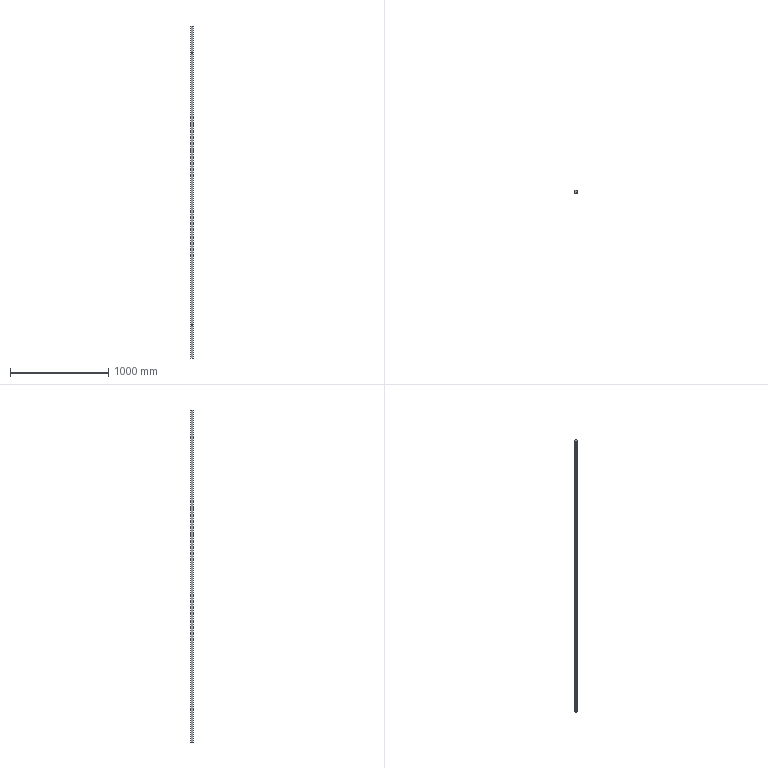Part | STEP file | BCC3 H16_8 | 1 solid | 14 faces | box 25 x 25 x 3385 mm | volume 2110006 mm3 | plane 10 | cylinder 4 | commonest cylinder face diameters 10 x4
STEP:
#1=CARTESIAN_POINT('',(0.,0.,0.));
#2=DIRECTION('',(0.,0.,1.));
#3=DIRECTION('',(1.,0.,0.));
#4=AXIS2_PLACEMENT_3D('',#1,#2,#3);
#5=CARTESIAN_POINT('',(0.,-12.5,-1347.5));
#6=VERTEX_POINT('',#5);
#7=CARTESIAN_POINT('',(0.,12.5,-1347.5));
#8=VERTEX_POINT('',#7);
#9=CARTESIAN_POINT('',(0.,-12.5,-1347.5));
#10=DIRECTION('',(0.,1.,0.));
#11=VECTOR('',#10,1.);
#12=LINE('',#9,#11);
#13=CARTESIAN_POINT('',(0.,-12.5,-1352.5));
#14=DIRECTION('',(0.,1.,0.));
#15=DIRECTION('',(0.,0.,1.));
#16=AXIS2_PLACEMENT_3D('',#13,#14,#15);
#17=CYLINDRICAL_SURFACE('',#16,5.);
#18=CARTESIAN_POINT('',(6.283,0.));
#19=DIRECTION('',(0.,1.));
#20=VECTOR('',#19,1.);
#21=LINE('',#18,#20);
#22=(GEOMETRIC_REPRESENTATION_CONTEXT(2)PARAMETRIC_REPRESENTATION_CONTEXT()REPRESENTATION_CONTEXT('',''));
#23=DEFINITIONAL_REPRESENTATION('',(#21),#22);
#24=PCURVE('',#17,#23);
#25=CARTESIAN_POINT('',(0.,-12.5,-1352.5));
#26=DIRECTION('',(0.,1.,0.));
#27=DIRECTION('',(0.,0.,1.));
#28=AXIS2_PLACEMENT_3D('',#25,#26,#27);
#29=CYLINDRICAL_SURFACE('',#28,5.);
#30=CARTESIAN_POINT('',(0.,0.));
#31=DIRECTION('',(0.,1.));
#32=VECTOR('',#31,1.);
#33=LINE('',#30,#32);
#34=(GEOMETRIC_REPRESENTATION_CONTEXT(2)PARAMETRIC_REPRESENTATION_CONTEXT()REPRESENTATION_CONTEXT('',''));
#35=DEFINITIONAL_REPRESENTATION('',(#33),#34);
#36=PCURVE('',#29,#35);
#37=SURFACE_CURVE('',#12,(#24,#36),.PCURVE_S1.);
#38=EDGE_CURVE('',#6,#8,#37,.T.);
#39=ORIENTED_EDGE('',*,*,#38,.T.);
#40=CARTESIAN_POINT('',(0.,12.5,-1357.5));
#41=VERTEX_POINT('',#40);
#42=CARTESIAN_POINT('',(0.,12.5,-1352.5));
#43=DIRECTION('',(0.,1.,0.));
#44=DIRECTION('',(0.,0.,1.));
#45=AXIS2_PLACEMENT_3D('',#42,#43,#44);
#46=CIRCLE('',#45,5.);
#47=CARTESIAN_POINT('',(0.,25.));
#48=DIRECTION('',(1.,0.));
#49=VECTOR('',#48,1.);
#50=LINE('',#47,#49);
#51=(GEOMETRIC_REPRESENTATION_CONTEXT(2)PARAMETRIC_REPRESENTATION_CONTEXT()REPRESENTATION_CONTEXT('',''));
#52=DEFINITIONAL_REPRESENTATION('',(#50),#51);
#53=PCURVE('',#17,#52);
#54=CARTESIAN_POINT('',(-12.5,12.5,1692.5));
#55=DIRECTION('',(0.,-1.,0.));
#56=DIRECTION('',(0.,0.,-1.));
#57=AXIS2_PLACEMENT_3D('',#54,#55,#56);
#58=PLANE('',#57);
#59=CARTESIAN_POINT('',(3040.,12.5));
#60=CARTESIAN_POINT('',(3040.,21.16));
#61=CARTESIAN_POINT('',(3047.5,16.83));
#62=CARTESIAN_POINT('',(3055.,12.5));
#63=CARTESIAN_POINT('',(3047.5,8.17));
#64=CARTESIAN_POINT('',(3040.,3.84));
#65=CARTESIAN_POINT('',(3040.,12.5));
#66=(BOUNDED_CURVE()B_SPLINE_CURVE(2,(#59,#60,#61,#62,#63,#64,#65),.UNSPECIFIED.,.T.,.F.)B_SPLINE_CURVE_WITH_KNOTS((1,2,2,2,2,1),(-2.094,0.,2.094,4.189,6.283,8.378),.UNSPECIFIED.)CURVE()GEOMETRIC_REPRESENTATION_ITEM()RATIONAL_B_SPLINE_CURVE((1.,0.5,1.,0.5,1.,0.5,1.))REPRESENTATION_ITEM(''));
#67=(GEOMETRIC_REPRESENTATION_CONTEXT(2)PARAMETRIC_REPRESENTATION_CONTEXT()REPRESENTATION_CONTEXT('',''));
#68=DEFINITIONAL_REPRESENTATION('',(#66),#67);
#69=PCURVE('',#58,#68);
#70=SURFACE_CURVE('',#46,(#53,#69),.PCURVE_S1.);
#71=EDGE_CURVE('',#41,#8,#70,.T.);
#72=ORIENTED_EDGE('',*,*,#71,.F.);
#73=CARTESIAN_POINT('',(0.,-12.5,-1357.5));
#74=VERTEX_POINT('',#73);
#75=CARTESIAN_POINT('',(0.,-12.5,-1357.5));
#76=DIRECTION('',(0.,1.,0.));
#77=VECTOR('',#76,1.);
#78=LINE('',#75,#77);
#79=CARTESIAN_POINT('',(3.142,0.));
#80=DIRECTION('',(0.,1.));
#81=VECTOR('',#80,1.);
#82=LINE('',#79,#81);
#83=(GEOMETRIC_REPRESENTATION_CONTEXT(2)PARAMETRIC_REPRESENTATION_CONTEXT()REPRESENTATION_CONTEXT('',''));
#84=DEFINITIONAL_REPRESENTATION('',(#82),#83);
#85=PCURVE('',#17,#84);
#86=CARTESIAN_POINT('',(3.142,0.));
#87=DIRECTION('',(0.,1.));
#88=VECTOR('',#87,1.);
#89=LINE('',#86,#88);
#90=(GEOMETRIC_REPRESENTATION_CONTEXT(2)PARAMETRIC_REPRESENTATION_CONTEXT()REPRESENTATION_CONTEXT('',''));
#91=DEFINITIONAL_REPRESENTATION('',(#89),#90);
#92=PCURVE('',#29,#91);
#93=SURFACE_CURVE('',#78,(#85,#92),.PCURVE_S1.);
#94=EDGE_CURVE('',#74,#41,#93,.T.);
#95=ORIENTED_EDGE('',*,*,#94,.F.);
#96=CARTESIAN_POINT('',(0.,-12.5,-1352.5));
#97=DIRECTION('',(0.,1.,0.));
#98=DIRECTION('',(0.,0.,1.));
#99=AXIS2_PLACEMENT_3D('',#96,#97,#98);
#100=CIRCLE('',#99,5.);
#101=CARTESIAN_POINT('',(0.,0.));
#102=DIRECTION('',(1.,0.));
#103=VECTOR('',#102,1.);
#104=LINE('',#101,#103);
#105=(GEOMETRIC_REPRESENTATION_CONTEXT(2)PARAMETRIC_REPRESENTATION_CONTEXT()REPRESENTATION_CONTEXT('',''));
#106=DEFINITIONAL_REPRESENTATION('',(#104),#105);
#107=PCURVE('',#17,#106);
#108=CARTESIAN_POINT('',(-12.5,-12.5,1692.5));
#109=DIRECTION('',(0.,1.,0.));
#110=DIRECTION('',(-1.,0.,0.));
#111=AXIS2_PLACEMENT_3D('',#108,#109,#110);
#112=PLANE('',#111);
#113=CARTESIAN_POINT('',(-12.5,-3045.));
#114=DIRECTION('',(0.,1.));
#115=AXIS2_PLACEMENT_2D('',#113,#114);
#116=CIRCLE('',#115,5.);
#117=(GEOMETRIC_REPRESENTATION_CONTEXT(2)PARAMETRIC_REPRESENTATION_CONTEXT()REPRESENTATION_CONTEXT('',''));
#118=DEFINITIONAL_REPRESENTATION('',(#116),#117);
#119=PCURVE('',#112,#118);
#120=SURFACE_CURVE('',#100,(#107,#119),.PCURVE_S1.);
#121=EDGE_CURVE('',#74,#6,#120,.T.);
#122=ORIENTED_EDGE('',*,*,#121,.T.);
#123=EDGE_LOOP('',(#39,#72,#95,#122));
#124=FACE_BOUND('',#123,.F.);
#125=ADVANCED_FACE('',(#124),#17,.F.);
#126=CARTESIAN_POINT('',(0.,-12.5,1422.5));
#127=VERTEX_POINT('',#126);
#128=CARTESIAN_POINT('',(0.,12.5,1422.5));
#129=VERTEX_POINT('',#128);
#130=CARTESIAN_POINT('',(0.,-12.5,1422.5));
#131=DIRECTION('',(0.,1.,0.));
#132=VECTOR('',#131,1.);
#133=LINE('',#130,#132);
#134=CARTESIAN_POINT('',(0.,-12.5,1417.5));
#135=DIRECTION('',(0.,1.,0.));
#136=DIRECTION('',(0.,0.,1.));
#137=AXIS2_PLACEMENT_3D('',#134,#135,#136);
#138=CYLINDRICAL_SURFACE('',#137,5.);
#139=CARTESIAN_POINT('',(6.283,0.));
#140=DIRECTION('',(0.,1.));
#141=VECTOR('',#140,1.);
#142=LINE('',#139,#141);
#143=(GEOMETRIC_REPRESENTATION_CONTEXT(2)PARAMETRIC_REPRESENTATION_CONTEXT()REPRESENTATION_CONTEXT('',''));
#144=DEFINITIONAL_REPRESENTATION('',(#142),#143);
#145=PCURVE('',#138,#144);
#146=CARTESIAN_POINT('',(0.,-12.5,1417.5));
#147=DIRECTION('',(0.,1.,0.));
#148=DIRECTION('',(0.,0.,1.));
#149=AXIS2_PLACEMENT_3D('',#146,#147,#148);
#150=CYLINDRICAL_SURFACE('',#149,5.);
#151=CARTESIAN_POINT('',(0.,0.));
#152=DIRECTION('',(0.,1.));
#153=VECTOR('',#152,1.);
#154=LINE('',#151,#153);
#155=(GEOMETRIC_REPRESENTATION_CONTEXT(2)PARAMETRIC_REPRESENTATION_CONTEXT()REPRESENTATION_CONTEXT('',''));
#156=DEFINITIONAL_REPRESENTATION('',(#154),#155);
#157=PCURVE('',#150,#156);
#158=SURFACE_CURVE('',#133,(#145,#157),.PCURVE_S1.);
#159=EDGE_CURVE('',#127,#129,#158,.T.);
#160=ORIENTED_EDGE('',*,*,#159,.T.);
#161=CARTESIAN_POINT('',(0.,12.5,1412.5));
#162=VERTEX_POINT('',#161);
#163=CARTESIAN_POINT('',(0.,12.5,1417.5));
#164=DIRECTION('',(0.,1.,0.));
#165=DIRECTION('',(0.,0.,1.));
#166=AXIS2_PLACEMENT_3D('',#163,#164,#165);
#167=CIRCLE('',#166,5.);
#168=CARTESIAN_POINT('',(0.,25.));
#169=DIRECTION('',(1.,0.));
#170=VECTOR('',#169,1.);
#171=LINE('',#168,#170);
#172=(GEOMETRIC_REPRESENTATION_CONTEXT(2)PARAMETRIC_REPRESENTATION_CONTEXT()REPRESENTATION_CONTEXT('',''));
#173=DEFINITIONAL_REPRESENTATION('',(#171),#172);
#174=PCURVE('',#138,#173);
#175=CARTESIAN_POINT('',(270.,12.5));
#176=CARTESIAN_POINT('',(270.,21.16));
#177=CARTESIAN_POINT('',(277.5,16.83));
#178=CARTESIAN_POINT('',(285.,12.5));
#179=CARTESIAN_POINT('',(277.5,8.17));
#180=CARTESIAN_POINT('',(270.,3.84));
#181=CARTESIAN_POINT('',(270.,12.5));
#182=(BOUNDED_CURVE()B_SPLINE_CURVE(2,(#175,#176,#177,#178,#179,#180,#181),.UNSPECIFIED.,.T.,.F.)B_SPLINE_CURVE_WITH_KNOTS((1,2,2,2,2,1),(-2.094,0.,2.094,4.189,6.283,8.378),.UNSPECIFIED.)CURVE()GEOMETRIC_REPRESENTATION_ITEM()RATIONAL_B_SPLINE_CURVE((1.,0.5,1.,0.5,1.,0.5,1.))REPRESENTATION_ITEM(''));
#183=(GEOMETRIC_REPRESENTATION_CONTEXT(2)PARAMETRIC_REPRESENTATION_CONTEXT()REPRESENTATION_CONTEXT('',''));
#184=DEFINITIONAL_REPRESENTATION('',(#182),#183);
#185=PCURVE('',#58,#184);
#186=SURFACE_CURVE('',#167,(#174,#185),.PCURVE_S1.);
#187=EDGE_CURVE('',#162,#129,#186,.T.);
#188=ORIENTED_EDGE('',*,*,#187,.F.);
#189=CARTESIAN_POINT('',(0.,-12.5,1412.5));
#190=VERTEX_POINT('',#189);
#191=CARTESIAN_POINT('',(0.,-12.5,1412.5));
#192=DIRECTION('',(0.,1.,0.));
#193=VECTOR('',#192,1.);
#194=LINE('',#191,#193);
#195=CARTESIAN_POINT('',(3.142,0.));
#196=DIRECTION('',(0.,1.));
#197=VECTOR('',#196,1.);
#198=LINE('',#195,#197);
#199=(GEOMETRIC_REPRESENTATION_CONTEXT(2)PARAMETRIC_REPRESENTATION_CONTEXT()REPRESENTATION_CONTEXT('',''));
#200=DEFINITIONAL_REPRESENTATION('',(#198),#199);
#201=PCURVE('',#138,#200);
#202=CARTESIAN_POINT('',(3.142,0.));
#203=DIRECTION('',(0.,1.));
#204=VECTOR('',#203,1.);
#205=LINE('',#202,#204);
#206=(GEOMETRIC_REPRESENTATION_CONTEXT(2)PARAMETRIC_REPRESENTATION_CONTEXT()REPRESENTATION_CONTEXT('',''));
#207=DEFINITIONAL_REPRESENTATION('',(#205),#206);
#208=PCURVE('',#150,#207);
#209=SURFACE_CURVE('',#194,(#201,#208),.PCURVE_S1.);
#210=EDGE_CURVE('',#190,#162,#209,.T.);
#211=ORIENTED_EDGE('',*,*,#210,.F.);
#212=CARTESIAN_POINT('',(0.,-12.5,1417.5));
#213=DIRECTION('',(0.,1.,0.));
#214=DIRECTION('',(0.,0.,1.));
#215=AXIS2_PLACEMENT_3D('',#212,#213,#214);
#216=CIRCLE('',#215,5.);
#217=CARTESIAN_POINT('',(0.,0.));
#218=DIRECTION('',(1.,0.));
#219=VECTOR('',#218,1.);
#220=LINE('',#217,#219);
#221=(GEOMETRIC_REPRESENTATION_CONTEXT(2)PARAMETRIC_REPRESENTATION_CONTEXT()REPRESENTATION_CONTEXT('',''));
#222=DEFINITIONAL_REPRESENTATION('',(#220),#221);
#223=PCURVE('',#138,#222);
#224=CARTESIAN_POINT('',(-12.5,-275.));
#225=DIRECTION('',(0.,1.));
#226=AXIS2_PLACEMENT_2D('',#224,#225);
#227=CIRCLE('',#226,5.);
#228=(GEOMETRIC_REPRESENTATION_CONTEXT(2)PARAMETRIC_REPRESENTATION_CONTEXT()REPRESENTATION_CONTEXT('',''));
#229=DEFINITIONAL_REPRESENTATION('',(#227),#228);
#230=PCURVE('',#112,#229);
#231=SURFACE_CURVE('',#216,(#223,#230),.PCURVE_S1.);
#232=EDGE_CURVE('',#190,#127,#231,.T.);
#233=ORIENTED_EDGE('',*,*,#232,.T.);
#234=EDGE_LOOP('',(#160,#188,#211,#233));
#235=FACE_BOUND('',#234,.F.);
#236=ADVANCED_FACE('',(#235),#138,.F.);
#237=CARTESIAN_POINT('',(-12.5,12.,-1692.5));
#238=VERTEX_POINT('',#237);
#239=CARTESIAN_POINT('',(-12.5,-12.,-1692.5));
#240=VERTEX_POINT('',#239);
#241=CARTESIAN_POINT('',(-12.5,12.5,-1692.5));
#242=DIRECTION('',(0.,-1.,0.));
#243=VECTOR('',#242,1.);
#244=LINE('',#241,#243);
#245=CARTESIAN_POINT('',(-12.5,12.5,1692.5));
#246=DIRECTION('',(1.,0.,0.));
#247=DIRECTION('',(0.,1.,0.));
#248=AXIS2_PLACEMENT_3D('',#245,#246,#247);
#249=PLANE('',#248);
#250=CARTESIAN_POINT('',(0.,-3385.));
#251=DIRECTION('',(-1.,0.));
#252=VECTOR('',#251,1.);
#253=LINE('',#250,#252);
#254=(GEOMETRIC_REPRESENTATION_CONTEXT(2)PARAMETRIC_REPRESENTATION_CONTEXT()REPRESENTATION_CONTEXT('',''));
#255=DEFINITIONAL_REPRESENTATION('',(#253),#254);
#256=PCURVE('',#249,#255);
#257=CARTESIAN_POINT('',(0.,0.,-1692.5));
#258=DIRECTION('',(0.,0.,1.));
#259=DIRECTION('',(1.,0.,0.));
#260=AXIS2_PLACEMENT_3D('',#257,#258,#259);
#261=PLANE('',#260);
#262=CARTESIAN_POINT('',(-12.5,12.5));
#263=DIRECTION('',(0.,-1.));
#264=VECTOR('',#263,1.);
#265=LINE('',#262,#264);
#266=(GEOMETRIC_REPRESENTATION_CONTEXT(2)PARAMETRIC_REPRESENTATION_CONTEXT()REPRESENTATION_CONTEXT('',''));
#267=DEFINITIONAL_REPRESENTATION('',(#265),#266);
#268=PCURVE('',#261,#267);
#269=SURFACE_CURVE('',#244,(#256,#268),.PCURVE_S1.);
#270=EDGE_CURVE('',#238,#240,#269,.T.);
#271=ORIENTED_EDGE('',*,*,#270,.T.);
#272=CARTESIAN_POINT('',(-12.5,-12.,1692.5));
#273=VERTEX_POINT('',#272);
#274=CARTESIAN_POINT('',(-12.5,-12.,1692.5));
#275=DIRECTION('',(0.,0.,1.));
#276=VECTOR('',#275,1.);
#277=LINE('',#274,#276);
#278=CARTESIAN_POINT('',(-24.5,0.));
#279=DIRECTION('',(0.,1.));
#280=VECTOR('',#279,1.);
#281=LINE('',#278,#280);
#282=(GEOMETRIC_REPRESENTATION_CONTEXT(2)PARAMETRIC_REPRESENTATION_CONTEXT()REPRESENTATION_CONTEXT('',''));
#283=DEFINITIONAL_REPRESENTATION('',(#281),#282);
#284=PCURVE('',#249,#283);
#285=CARTESIAN_POINT('',(-12.,-12.5,1692.5));
#286=DIRECTION('',(0.7071,0.7071,0.));
#287=DIRECTION('',(0.,0.,-1.));
#288=AXIS2_PLACEMENT_3D('',#285,#286,#287);
#289=PLANE('',#288);
#290=CARTESIAN_POINT('',(0.,0.7071));
#291=DIRECTION('',(-1.,0.));
#292=VECTOR('',#291,1.);
#293=LINE('',#290,#292);
#294=(GEOMETRIC_REPRESENTATION_CONTEXT(2)PARAMETRIC_REPRESENTATION_CONTEXT()REPRESENTATION_CONTEXT('',''));
#295=DEFINITIONAL_REPRESENTATION('',(#293),#294);
#296=PCURVE('',#289,#295);
#297=SURFACE_CURVE('',#277,(#284,#296),.PCURVE_S1.);
#298=EDGE_CURVE('',#240,#273,#297,.T.);
#299=ORIENTED_EDGE('',*,*,#298,.T.);
#300=CARTESIAN_POINT('',(-12.5,12.,1692.5));
#301=VERTEX_POINT('',#300);
#302=CARTESIAN_POINT('',(-12.5,12.5,1692.5));
#303=DIRECTION('',(0.,-1.,0.));
#304=VECTOR('',#303,1.);
#305=LINE('',#302,#304);
#306=CARTESIAN_POINT('',(0.,0.));
#307=DIRECTION('',(-1.,0.));
#308=VECTOR('',#307,1.);
#309=LINE('',#306,#308);
#310=(GEOMETRIC_REPRESENTATION_CONTEXT(2)PARAMETRIC_REPRESENTATION_CONTEXT()REPRESENTATION_CONTEXT('',''));
#311=DEFINITIONAL_REPRESENTATION('',(#309),#310);
#312=PCURVE('',#249,#311);
#313=CARTESIAN_POINT('',(0.,0.,1692.5));
#314=DIRECTION('',(0.,0.,1.));
#315=DIRECTION('',(1.,0.,0.));
#316=AXIS2_PLACEMENT_3D('',#313,#314,#315);
#317=PLANE('',#316);
#318=CARTESIAN_POINT('',(-12.5,12.5));
#319=DIRECTION('',(0.,-1.));
#320=VECTOR('',#319,1.);
#321=LINE('',#318,#320);
#322=(GEOMETRIC_REPRESENTATION_CONTEXT(2)PARAMETRIC_REPRESENTATION_CONTEXT()REPRESENTATION_CONTEXT('',''));
#323=DEFINITIONAL_REPRESENTATION('',(#321),#322);
#324=PCURVE('',#317,#323);
#325=SURFACE_CURVE('',#305,(#312,#324),.PCURVE_S1.);
#326=EDGE_CURVE('',#301,#273,#325,.T.);
#327=ORIENTED_EDGE('',*,*,#326,.F.);
#328=CARTESIAN_POINT('',(-12.5,12.,1692.5));
#329=DIRECTION('',(0.,0.,-1.));
#330=VECTOR('',#329,1.);
#331=LINE('',#328,#330);
#332=CARTESIAN_POINT('',(-0.5,0.));
#333=DIRECTION('',(0.,-1.));
#334=VECTOR('',#333,1.);
#335=LINE('',#332,#334);
#336=(GEOMETRIC_REPRESENTATION_CONTEXT(2)PARAMETRIC_REPRESENTATION_CONTEXT()REPRESENTATION_CONTEXT('',''));
#337=DEFINITIONAL_REPRESENTATION('',(#335),#336);
#338=PCURVE('',#249,#337);
#339=CARTESIAN_POINT('',(-12.5,12.,1692.5));
#340=DIRECTION('',(0.7071,-0.7071,0.));
#341=DIRECTION('',(0.,0.,-1.));
#342=AXIS2_PLACEMENT_3D('',#339,#340,#341);
#343=PLANE('',#342);
#344=CARTESIAN_POINT('',(0.,0.));
#345=DIRECTION('',(1.,0.));
#346=VECTOR('',#345,1.);
#347=LINE('',#344,#346);
#348=(GEOMETRIC_REPRESENTATION_CONTEXT(2)PARAMETRIC_REPRESENTATION_CONTEXT()REPRESENTATION_CONTEXT('',''));
#349=DEFINITIONAL_REPRESENTATION('',(#347),#348);
#350=PCURVE('',#343,#349);
#351=SURFACE_CURVE('',#331,(#338,#350),.PCURVE_S1.);
#352=EDGE_CURVE('',#301,#238,#351,.T.);
#353=ORIENTED_EDGE('',*,*,#352,.T.);
#354=EDGE_LOOP('',(#271,#299,#327,#353));
#355=FACE_BOUND('',#354,.T.);
#356=ADVANCED_FACE('',(#355),#249,.F.);
#357=CARTESIAN_POINT('',(0.,-12.5,-1352.5));
#358=DIRECTION('',(0.,1.,0.));
#359=DIRECTION('',(0.,0.,1.));
#360=AXIS2_PLACEMENT_3D('',#357,#358,#359);
#361=CIRCLE('',#360,5.);
#362=CARTESIAN_POINT('',(-12.5,-3045.));
#363=DIRECTION('',(0.,1.));
#364=AXIS2_PLACEMENT_2D('',#362,#363);
#365=CIRCLE('',#364,5.);
#366=(GEOMETRIC_REPRESENTATION_CONTEXT(2)PARAMETRIC_REPRESENTATION_CONTEXT()REPRESENTATION_CONTEXT('',''));
#367=DEFINITIONAL_REPRESENTATION('',(#365),#366);
#368=PCURVE('',#112,#367);
#369=CARTESIAN_POINT('',(0.,0.));
#370=DIRECTION('',(1.,0.));
#371=VECTOR('',#370,1.);
#372=LINE('',#369,#371);
#373=(GEOMETRIC_REPRESENTATION_CONTEXT(2)PARAMETRIC_REPRESENTATION_CONTEXT()REPRESENTATION_CONTEXT('',''));
#374=DEFINITIONAL_REPRESENTATION('',(#372),#373);
#375=PCURVE('',#29,#374);
#376=SURFACE_CURVE('',#361,(#368,#375),.PCURVE_S1.);
#377=EDGE_CURVE('',#6,#74,#376,.T.);
#378=ORIENTED_EDGE('',*,*,#377,.T.);
#379=ORIENTED_EDGE('',*,*,#121,.T.);
#380=EDGE_LOOP('',(#378,#379));
#381=FACE_BOUND('',#380,.T.);
#382=CARTESIAN_POINT('',(0.,-12.5,1417.5));
#383=DIRECTION('',(0.,1.,0.));
#384=DIRECTION('',(0.,0.,1.));
#385=AXIS2_PLACEMENT_3D('',#382,#383,#384);
#386=CIRCLE('',#385,5.);
#387=CARTESIAN_POINT('',(-12.5,-275.));
#388=DIRECTION('',(0.,1.));
#389=AXIS2_PLACEMENT_2D('',#387,#388);
#390=CIRCLE('',#389,5.);
#391=(GEOMETRIC_REPRESENTATION_CONTEXT(2)PARAMETRIC_REPRESENTATION_CONTEXT()REPRESENTATION_CONTEXT('',''));
#392=DEFINITIONAL_REPRESENTATION('',(#390),#391);
#393=PCURVE('',#112,#392);
#394=CARTESIAN_POINT('',(0.,0.));
#395=DIRECTION('',(1.,0.));
#396=VECTOR('',#395,1.);
#397=LINE('',#394,#396);
#398=(GEOMETRIC_REPRESENTATION_CONTEXT(2)PARAMETRIC_REPRESENTATION_CONTEXT()REPRESENTATION_CONTEXT('',''));
#399=DEFINITIONAL_REPRESENTATION('',(#397),#398);
#400=PCURVE('',#150,#399);
#401=SURFACE_CURVE('',#386,(#393,#400),.PCURVE_S1.);
#402=EDGE_CURVE('',#127,#190,#401,.T.);
#403=ORIENTED_EDGE('',*,*,#402,.T.);
#404=ORIENTED_EDGE('',*,*,#232,.T.);
#405=EDGE_LOOP('',(#403,#404));
#406=FACE_BOUND('',#405,.T.);
#407=CARTESIAN_POINT('',(-12.,-12.5,1692.5));
#408=VERTEX_POINT('',#407);
#409=CARTESIAN_POINT('',(12.,-12.5,1692.5));
#410=VERTEX_POINT('',#409);
#411=CARTESIAN_POINT('',(-12.5,-12.5,1692.5));
#412=DIRECTION('',(1.,0.,0.));
#413=VECTOR('',#412,1.);
#414=LINE('',#411,#413);
#415=CARTESIAN_POINT('',(0.,0.));
#416=DIRECTION('',(-1.,0.));
#417=VECTOR('',#416,1.);
#418=LINE('',#415,#417);
#419=(GEOMETRIC_REPRESENTATION_CONTEXT(2)PARAMETRIC_REPRESENTATION_CONTEXT()REPRESENTATION_CONTEXT('',''));
#420=DEFINITIONAL_REPRESENTATION('',(#418),#419);
#421=PCURVE('',#112,#420);
#422=CARTESIAN_POINT('',(-12.5,-12.5));
#423=DIRECTION('',(1.,0.));
#424=VECTOR('',#423,1.);
#425=LINE('',#422,#424);
#426=(GEOMETRIC_REPRESENTATION_CONTEXT(2)PARAMETRIC_REPRESENTATION_CONTEXT()REPRESENTATION_CONTEXT('',''));
#427=DEFINITIONAL_REPRESENTATION('',(#425),#426);
#428=PCURVE('',#317,#427);
#429=SURFACE_CURVE('',#414,(#421,#428),.PCURVE_S1.);
#430=EDGE_CURVE('',#408,#410,#429,.T.);
#431=ORIENTED_EDGE('',*,*,#430,.F.);
#432=CARTESIAN_POINT('',(-12.,-12.5,-1692.5));
#433=VERTEX_POINT('',#432);
#434=CARTESIAN_POINT('',(-12.,-12.5,1692.5));
#435=DIRECTION('',(0.,0.,-1.));
#436=VECTOR('',#435,1.);
#437=LINE('',#434,#436);
#438=CARTESIAN_POINT('',(-0.5,0.));
#439=DIRECTION('',(0.,-1.));
#440=VECTOR('',#439,1.);
#441=LINE('',#438,#440);
#442=(GEOMETRIC_REPRESENTATION_CONTEXT(2)PARAMETRIC_REPRESENTATION_CONTEXT()REPRESENTATION_CONTEXT('',''));
#443=DEFINITIONAL_REPRESENTATION('',(#441),#442);
#444=PCURVE('',#112,#443);
#445=CARTESIAN_POINT('',(0.,0.));
#446=DIRECTION('',(1.,0.));
#447=VECTOR('',#446,1.);
#448=LINE('',#445,#447);
#449=(GEOMETRIC_REPRESENTATION_CONTEXT(2)PARAMETRIC_REPRESENTATION_CONTEXT()REPRESENTATION_CONTEXT('',''));
#450=DEFINITIONAL_REPRESENTATION('',(#448),#449);
#451=PCURVE('',#289,#450);
#452=SURFACE_CURVE('',#437,(#444,#451),.PCURVE_S1.);
#453=EDGE_CURVE('',#408,#433,#452,.T.);
#454=ORIENTED_EDGE('',*,*,#453,.T.);
#455=CARTESIAN_POINT('',(12.,-12.5,-1692.5));
#456=VERTEX_POINT('',#455);
#457=CARTESIAN_POINT('',(-12.5,-12.5,-1692.5));
#458=DIRECTION('',(1.,0.,0.));
#459=VECTOR('',#458,1.);
#460=LINE('',#457,#459);
#461=CARTESIAN_POINT('',(0.,-3385.));
#462=DIRECTION('',(-1.,0.));
#463=VECTOR('',#462,1.);
#464=LINE('',#461,#463);
#465=(GEOMETRIC_REPRESENTATION_CONTEXT(2)PARAMETRIC_REPRESENTATION_CONTEXT()REPRESENTATION_CONTEXT('',''));
#466=DEFINITIONAL_REPRESENTATION('',(#464),#465);
#467=PCURVE('',#112,#466);
#468=CARTESIAN_POINT('',(-12.5,-12.5));
#469=DIRECTION('',(1.,0.));
#470=VECTOR('',#469,1.);
#471=LINE('',#468,#470);
#472=(GEOMETRIC_REPRESENTATION_CONTEXT(2)PARAMETRIC_REPRESENTATION_CONTEXT()REPRESENTATION_CONTEXT('',''));
#473=DEFINITIONAL_REPRESENTATION('',(#471),#472);
#474=PCURVE('',#261,#473);
#475=SURFACE_CURVE('',#460,(#467,#474),.PCURVE_S1.);
#476=EDGE_CURVE('',#433,#456,#475,.T.);
#477=ORIENTED_EDGE('',*,*,#476,.T.);
#478=CARTESIAN_POINT('',(12.,-12.5,1692.5));
#479=DIRECTION('',(0.,0.,1.));
#480=VECTOR('',#479,1.);
#481=LINE('',#478,#480);
#482=CARTESIAN_POINT('',(-24.5,0.));
#483=DIRECTION('',(0.,1.));
#484=VECTOR('',#483,1.);
#485=LINE('',#482,#484);
#486=(GEOMETRIC_REPRESENTATION_CONTEXT(2)PARAMETRIC_REPRESENTATION_CONTEXT()REPRESENTATION_CONTEXT('',''));
#487=DEFINITIONAL_REPRESENTATION('',(#485),#486);
#488=PCURVE('',#112,#487);
#489=CARTESIAN_POINT('',(12.5,-12.,1692.5));
#490=DIRECTION('',(-0.7071,0.7071,0.));
#491=DIRECTION('',(0.,0.,-1.));
#492=AXIS2_PLACEMENT_3D('',#489,#490,#491);
#493=PLANE('',#492);
#494=CARTESIAN_POINT('',(0.,0.7071));
#495=DIRECTION('',(-1.,0.));
#496=VECTOR('',#495,1.);
#497=LINE('',#494,#496);
#498=(GEOMETRIC_REPRESENTATION_CONTEXT(2)PARAMETRIC_REPRESENTATION_CONTEXT()REPRESENTATION_CONTEXT('',''));
#499=DEFINITIONAL_REPRESENTATION('',(#497),#498);
#500=PCURVE('',#493,#499);
#501=SURFACE_CURVE('',#481,(#488,#500),.PCURVE_S1.);
#502=EDGE_CURVE('',#456,#410,#501,.T.);
#503=ORIENTED_EDGE('',*,*,#502,.T.);
#504=EDGE_LOOP('',(#431,#454,#477,#503));
#505=FACE_BOUND('',#504,.T.);
#506=ADVANCED_FACE('',(#381,#406,#505),#112,.F.);
#507=CARTESIAN_POINT('',(12.5,-12.,1692.5));
#508=VERTEX_POINT('',#507);
#509=CARTESIAN_POINT('',(12.5,12.,1692.5));
#510=VERTEX_POINT('',#509);
#511=CARTESIAN_POINT('',(12.5,12.5,1692.5));
#512=DIRECTION('',(0.,1.,0.));
#513=VECTOR('',#512,1.);
#514=LINE('',#511,#513);
#515=CARTESIAN_POINT('',(12.5,12.5,1692.5));
#516=DIRECTION('',(-1.,0.,0.));
#517=DIRECTION('',(0.,-1.,0.));
#518=AXIS2_PLACEMENT_3D('',#515,#516,#517);
#519=PLANE('',#518);
#520=CARTESIAN_POINT('',(0.,0.));
#521=DIRECTION('',(-1.,0.));
#522=VECTOR('',#521,1.);
#523=LINE('',#520,#522);
#524=(GEOMETRIC_REPRESENTATION_CONTEXT(2)PARAMETRIC_REPRESENTATION_CONTEXT()REPRESENTATION_CONTEXT('',''));
#525=DEFINITIONAL_REPRESENTATION('',(#523),#524);
#526=PCURVE('',#519,#525);
#527=CARTESIAN_POINT('',(12.5,12.5));
#528=DIRECTION('',(0.,1.));
#529=VECTOR('',#528,1.);
#530=LINE('',#527,#529);
#531=(GEOMETRIC_REPRESENTATION_CONTEXT(2)PARAMETRIC_REPRESENTATION_CONTEXT()REPRESENTATION_CONTEXT('',''));
#532=DEFINITIONAL_REPRESENTATION('',(#530),#531);
#533=PCURVE('',#317,#532);
#534=SURFACE_CURVE('',#514,(#526,#533),.PCURVE_S1.);
#535=EDGE_CURVE('',#508,#510,#534,.T.);
#536=ORIENTED_EDGE('',*,*,#535,.F.);
#537=CARTESIAN_POINT('',(12.5,-12.,-1692.5));
#538=VERTEX_POINT('',#537);
#539=CARTESIAN_POINT('',(12.5,-12.,1692.5));
#540=DIRECTION('',(0.,0.,-1.));
#541=VECTOR('',#540,1.);
#542=LINE('',#539,#541);
#543=CARTESIAN_POINT('',(24.5,0.));
#544=DIRECTION('',(0.,-1.));
#545=VECTOR('',#544,1.);
#546=LINE('',#543,#545);
#547=(GEOMETRIC_REPRESENTATION_CONTEXT(2)PARAMETRIC_REPRESENTATION_CONTEXT()REPRESENTATION_CONTEXT('',''));
#548=DEFINITIONAL_REPRESENTATION('',(#546),#547);
#549=PCURVE('',#519,#548);
#550=CARTESIAN_POINT('',(0.,0.));
#551=DIRECTION('',(1.,0.));
#552=VECTOR('',#551,1.);
#553=LINE('',#550,#552);
#554=(GEOMETRIC_REPRESENTATION_CONTEXT(2)PARAMETRIC_REPRESENTATION_CONTEXT()REPRESENTATION_CONTEXT('',''));
#555=DEFINITIONAL_REPRESENTATION('',(#553),#554);
#556=PCURVE('',#493,#555);
#557=SURFACE_CURVE('',#542,(#549,#556),.PCURVE_S1.);
#558=EDGE_CURVE('',#508,#538,#557,.T.);
#559=ORIENTED_EDGE('',*,*,#558,.T.);
#560=CARTESIAN_POINT('',(12.5,12.,-1692.5));
#561=VERTEX_POINT('',#560);
#562=CARTESIAN_POINT('',(12.5,12.5,-1692.5));
#563=DIRECTION('',(0.,1.,0.));
#564=VECTOR('',#563,1.);
#565=LINE('',#562,#564);
#566=CARTESIAN_POINT('',(0.,-3385.));
#567=DIRECTION('',(-1.,0.));
#568=VECTOR('',#567,1.);
#569=LINE('',#566,#568);
#570=(GEOMETRIC_REPRESENTATION_CONTEXT(2)PARAMETRIC_REPRESENTATION_CONTEXT()REPRESENTATION_CONTEXT('',''));
#571=DEFINITIONAL_REPRESENTATION('',(#569),#570);
#572=PCURVE('',#519,#571);
#573=CARTESIAN_POINT('',(12.5,12.5));
#574=DIRECTION('',(0.,1.));
#575=VECTOR('',#574,1.);
#576=LINE('',#573,#575);
#577=(GEOMETRIC_REPRESENTATION_CONTEXT(2)PARAMETRIC_REPRESENTATION_CONTEXT()REPRESENTATION_CONTEXT('',''));
#578=DEFINITIONAL_REPRESENTATION('',(#576),#577);
#579=PCURVE('',#261,#578);
#580=SURFACE_CURVE('',#565,(#572,#579),.PCURVE_S1.);
#581=EDGE_CURVE('',#538,#561,#580,.T.);
#582=ORIENTED_EDGE('',*,*,#581,.T.);
#583=CARTESIAN_POINT('',(12.5,12.,1692.5));
#584=DIRECTION('',(0.,0.,1.));
#585=VECTOR('',#584,1.);
#586=LINE('',#583,#585);
#587=CARTESIAN_POINT('',(0.5,0.));
#588=DIRECTION('',(0.,1.));
#589=VECTOR('',#588,1.);
#590=LINE('',#587,#589);
#591=(GEOMETRIC_REPRESENTATION_CONTEXT(2)PARAMETRIC_REPRESENTATION_CONTEXT()REPRESENTATION_CONTEXT('',''));
#592=DEFINITIONAL_REPRESENTATION('',(#590),#591);
#593=PCURVE('',#519,#592);
#594=CARTESIAN_POINT('',(12.,12.5,1692.5));
#595=DIRECTION('',(-0.7071,-0.7071,0.));
#596=DIRECTION('',(0.,0.,-1.));
#597=AXIS2_PLACEMENT_3D('',#594,#595,#596);
#598=PLANE('',#597);
#599=CARTESIAN_POINT('',(0.,0.7071));
#600=DIRECTION('',(-1.,0.));
#601=VECTOR('',#600,1.);
#602=LINE('',#599,#601);
#603=(GEOMETRIC_REPRESENTATION_CONTEXT(2)PARAMETRIC_REPRESENTATION_CONTEXT()REPRESENTATION_CONTEXT('',''));
#604=DEFINITIONAL_REPRESENTATION('',(#602),#603);
#605=PCURVE('',#598,#604);
#606=SURFACE_CURVE('',#586,(#593,#605),.PCURVE_S1.);
#607=EDGE_CURVE('',#561,#510,#606,.T.);
#608=ORIENTED_EDGE('',*,*,#607,.T.);
#609=EDGE_LOOP('',(#536,#559,#582,#608));
#610=FACE_BOUND('',#609,.T.);
#611=ADVANCED_FACE('',(#610),#519,.F.);
#612=CARTESIAN_POINT('',(0.,12.5,-1352.5));
#613=DIRECTION('',(0.,1.,0.));
#614=DIRECTION('',(0.,0.,1.));
#615=AXIS2_PLACEMENT_3D('',#612,#613,#614);
#616=CIRCLE('',#615,5.);
#617=CARTESIAN_POINT('',(3040.,12.5));
#618=CARTESIAN_POINT('',(3040.,21.16));
#619=CARTESIAN_POINT('',(3047.5,16.83));
#620=CARTESIAN_POINT('',(3055.,12.5));
#621=CARTESIAN_POINT('',(3047.5,8.17));
#622=CARTESIAN_POINT('',(3040.,3.84));
#623=CARTESIAN_POINT('',(3040.,12.5));
#624=(BOUNDED_CURVE()B_SPLINE_CURVE(2,(#617,#618,#619,#620,#621,#622,#623),.UNSPECIFIED.,.T.,.F.)B_SPLINE_CURVE_WITH_KNOTS((1,2,2,2,2,1),(-2.094,0.,2.094,4.189,6.283,8.378),.UNSPECIFIED.)CURVE()GEOMETRIC_REPRESENTATION_ITEM()RATIONAL_B_SPLINE_CURVE((1.,0.5,1.,0.5,1.,0.5,1.))REPRESENTATION_ITEM(''));
#625=(GEOMETRIC_REPRESENTATION_CONTEXT(2)PARAMETRIC_REPRESENTATION_CONTEXT()REPRESENTATION_CONTEXT('',''));
#626=DEFINITIONAL_REPRESENTATION('',(#624),#625);
#627=PCURVE('',#58,#626);
#628=CARTESIAN_POINT('',(0.,25.));
#629=DIRECTION('',(1.,0.));
#630=VECTOR('',#629,1.);
#631=LINE('',#628,#630);
#632=(GEOMETRIC_REPRESENTATION_CONTEXT(2)PARAMETRIC_REPRESENTATION_CONTEXT()REPRESENTATION_CONTEXT('',''));
#633=DEFINITIONAL_REPRESENTATION('',(#631),#632);
#634=PCURVE('',#29,#633);
#635=SURFACE_CURVE('',#616,(#627,#634),.PCURVE_S1.);
#636=EDGE_CURVE('',#8,#41,#635,.T.);
#637=ORIENTED_EDGE('',*,*,#636,.F.);
#638=ORIENTED_EDGE('',*,*,#71,.F.);
#639=EDGE_LOOP('',(#637,#638));
#640=FACE_BOUND('',#639,.T.);
#641=CARTESIAN_POINT('',(0.,12.5,1417.5));
#642=DIRECTION('',(0.,1.,0.));
#643=DIRECTION('',(0.,0.,1.));
#644=AXIS2_PLACEMENT_3D('',#641,#642,#643);
#645=CIRCLE('',#644,5.);
#646=CARTESIAN_POINT('',(270.,12.5));
#647=CARTESIAN_POINT('',(270.,21.16));
#648=CARTESIAN_POINT('',(277.5,16.83));
#649=CARTESIAN_POINT('',(285.,12.5));
#650=CARTESIAN_POINT('',(277.5,8.17));
#651=CARTESIAN_POINT('',(270.,3.84));
#652=CARTESIAN_POINT('',(270.,12.5));
#653=(BOUNDED_CURVE()B_SPLINE_CURVE(2,(#646,#647,#648,#649,#650,#651,#652),.UNSPECIFIED.,.T.,.F.)B_SPLINE_CURVE_WITH_KNOTS((1,2,2,2,2,1),(-2.094,0.,2.094,4.189,6.283,8.378),.UNSPECIFIED.)CURVE()GEOMETRIC_REPRESENTATION_ITEM()RATIONAL_B_SPLINE_CURVE((1.,0.5,1.,0.5,1.,0.5,1.))REPRESENTATION_ITEM(''));
#654=(GEOMETRIC_REPRESENTATION_CONTEXT(2)PARAMETRIC_REPRESENTATION_CONTEXT()REPRESENTATION_CONTEXT('',''));
#655=DEFINITIONAL_REPRESENTATION('',(#653),#654);
#656=PCURVE('',#58,#655);
#657=CARTESIAN_POINT('',(0.,25.));
#658=DIRECTION('',(1.,0.));
#659=VECTOR('',#658,1.);
#660=LINE('',#657,#659);
#661=(GEOMETRIC_REPRESENTATION_CONTEXT(2)PARAMETRIC_REPRESENTATION_CONTEXT()REPRESENTATION_CONTEXT('',''));
#662=DEFINITIONAL_REPRESENTATION('',(#660),#661);
#663=PCURVE('',#150,#662);
#664=SURFACE_CURVE('',#645,(#656,#663),.PCURVE_S1.);
#665=EDGE_CURVE('',#129,#162,#664,.T.);
#666=ORIENTED_EDGE('',*,*,#665,.F.);
#667=ORIENTED_EDGE('',*,*,#187,.F.);
#668=EDGE_LOOP('',(#666,#667));
#669=FACE_BOUND('',#668,.T.);
#670=CARTESIAN_POINT('',(12.,12.5,-1692.5));
#671=VERTEX_POINT('',#670);
#672=CARTESIAN_POINT('',(-12.,12.5,-1692.5));
#673=VERTEX_POINT('',#672);
#674=CARTESIAN_POINT('',(-12.5,12.5,-1692.5));
#675=DIRECTION('',(-1.,0.,0.));
#676=VECTOR('',#675,1.);
#677=LINE('',#674,#676);
#678=CARTESIAN_POINT('',(3385.,0.));
#679=DIRECTION('',(0.,-1.));
#680=VECTOR('',#679,1.);
#681=LINE('',#678,#680);
#682=(GEOMETRIC_REPRESENTATION_CONTEXT(2)PARAMETRIC_REPRESENTATION_CONTEXT()REPRESENTATION_CONTEXT('',''));
#683=DEFINITIONAL_REPRESENTATION('',(#681),#682);
#684=PCURVE('',#58,#683);
#685=CARTESIAN_POINT('',(-12.5,12.5));
#686=DIRECTION('',(-1.,0.));
#687=VECTOR('',#686,1.);
#688=LINE('',#685,#687);
#689=(GEOMETRIC_REPRESENTATION_CONTEXT(2)PARAMETRIC_REPRESENTATION_CONTEXT()REPRESENTATION_CONTEXT('',''));
#690=DEFINITIONAL_REPRESENTATION('',(#688),#689);
#691=PCURVE('',#261,#690);
#692=SURFACE_CURVE('',#677,(#684,#691),.PCURVE_S1.);
#693=EDGE_CURVE('',#671,#673,#692,.T.);
#694=ORIENTED_EDGE('',*,*,#693,.T.);
#695=CARTESIAN_POINT('',(-12.,12.5,1692.5));
#696=VERTEX_POINT('',#695);
#697=CARTESIAN_POINT('',(-12.,12.5,1692.5));
#698=DIRECTION('',(0.,0.,1.));
#699=VECTOR('',#698,1.);
#700=LINE('',#697,#699);
#701=CARTESIAN_POINT('',(0.,0.5));
#702=DIRECTION('',(-1.,0.));
#703=VECTOR('',#702,1.);
#704=LINE('',#701,#703);
#705=(GEOMETRIC_REPRESENTATION_CONTEXT(2)PARAMETRIC_REPRESENTATION_CONTEXT()REPRESENTATION_CONTEXT('',''));
#706=DEFINITIONAL_REPRESENTATION('',(#704),#705);
#707=PCURVE('',#58,#706);
#708=CARTESIAN_POINT('',(0.,0.7071));
#709=DIRECTION('',(-1.,0.));
#710=VECTOR('',#709,1.);
#711=LINE('',#708,#710);
#712=(GEOMETRIC_REPRESENTATION_CONTEXT(2)PARAMETRIC_REPRESENTATION_CONTEXT()REPRESENTATION_CONTEXT('',''));
#713=DEFINITIONAL_REPRESENTATION('',(#711),#712);
#714=PCURVE('',#343,#713);
#715=SURFACE_CURVE('',#700,(#707,#714),.PCURVE_S1.);
#716=EDGE_CURVE('',#673,#696,#715,.T.);
#717=ORIENTED_EDGE('',*,*,#716,.T.);
#718=CARTESIAN_POINT('',(12.,12.5,1692.5));
#719=VERTEX_POINT('',#718);
#720=CARTESIAN_POINT('',(-12.5,12.5,1692.5));
#721=DIRECTION('',(-1.,0.,0.));
#722=VECTOR('',#721,1.);
#723=LINE('',#720,#722);
#724=CARTESIAN_POINT('',(0.,0.));
#725=DIRECTION('',(0.,-1.));
#726=VECTOR('',#725,1.);
#727=LINE('',#724,#726);
#728=(GEOMETRIC_REPRESENTATION_CONTEXT(2)PARAMETRIC_REPRESENTATION_CONTEXT()REPRESENTATION_CONTEXT('',''));
#729=DEFINITIONAL_REPRESENTATION('',(#727),#728);
#730=PCURVE('',#58,#729);
#731=CARTESIAN_POINT('',(-12.5,12.5));
#732=DIRECTION('',(-1.,0.));
#733=VECTOR('',#732,1.);
#734=LINE('',#731,#733);
#735=(GEOMETRIC_REPRESENTATION_CONTEXT(2)PARAMETRIC_REPRESENTATION_CONTEXT()REPRESENTATION_CONTEXT('',''));
#736=DEFINITIONAL_REPRESENTATION('',(#734),#735);
#737=PCURVE('',#317,#736);
#738=SURFACE_CURVE('',#723,(#730,#737),.PCURVE_S1.);
#739=EDGE_CURVE('',#719,#696,#738,.T.);
#740=ORIENTED_EDGE('',*,*,#739,.F.);
#741=CARTESIAN_POINT('',(12.,12.5,1692.5));
#742=DIRECTION('',(0.,0.,-1.));
#743=VECTOR('',#742,1.);
#744=LINE('',#741,#743);
#745=CARTESIAN_POINT('',(0.,24.5));
#746=DIRECTION('',(1.,0.));
#747=VECTOR('',#746,1.);
#748=LINE('',#745,#747);
#749=(GEOMETRIC_REPRESENTATION_CONTEXT(2)PARAMETRIC_REPRESENTATION_CONTEXT()REPRESENTATION_CONTEXT('',''));
#750=DEFINITIONAL_REPRESENTATION('',(#748),#749);
#751=PCURVE('',#58,#750);
#752=CARTESIAN_POINT('',(0.,0.));
#753=DIRECTION('',(1.,0.));
#754=VECTOR('',#753,1.);
#755=LINE('',#752,#754);
#756=(GEOMETRIC_REPRESENTATION_CONTEXT(2)PARAMETRIC_REPRESENTATION_CONTEXT()REPRESENTATION_CONTEXT('',''));
#757=DEFINITIONAL_REPRESENTATION('',(#755),#756);
#758=PCURVE('',#598,#757);
#759=SURFACE_CURVE('',#744,(#751,#758),.PCURVE_S1.);
#760=EDGE_CURVE('',#719,#671,#759,.T.);
#761=ORIENTED_EDGE('',*,*,#760,.T.);
#762=EDGE_LOOP('',(#694,#717,#740,#761));
#763=FACE_BOUND('',#762,.T.);
#764=ADVANCED_FACE('',(#640,#669,#763),#58,.F.);
#765=ORIENTED_EDGE('',*,*,#326,.T.);
#766=CARTESIAN_POINT('',(-12.25,-12.25,1692.5));
#767=DIRECTION('',(0.7071,-0.7071,0.));
#768=VECTOR('',#767,1.);
#769=LINE('',#766,#768);
#770=CARTESIAN_POINT('',(-12.25,-12.25));
#771=DIRECTION('',(0.7071,-0.7071));
#772=VECTOR('',#771,1.);
#773=LINE('',#770,#772);
#774=(GEOMETRIC_REPRESENTATION_CONTEXT(2)PARAMETRIC_REPRESENTATION_CONTEXT()REPRESENTATION_CONTEXT('',''));
#775=DEFINITIONAL_REPRESENTATION('',(#773),#774);
#776=PCURVE('',#317,#775);
#777=CARTESIAN_POINT('',(0.,0.3536));
#778=DIRECTION('',(0.,-1.));
#779=VECTOR('',#778,1.);
#780=LINE('',#777,#779);
#781=(GEOMETRIC_REPRESENTATION_CONTEXT(2)PARAMETRIC_REPRESENTATION_CONTEXT()REPRESENTATION_CONTEXT('',''));
#782=DEFINITIONAL_REPRESENTATION('',(#780),#781);
#783=PCURVE('',#289,#782);
#784=SURFACE_CURVE('',#769,(#776,#783),.PCURVE_S1.);
#785=EDGE_CURVE('',#273,#408,#784,.T.);
#786=ORIENTED_EDGE('',*,*,#785,.T.);
#787=ORIENTED_EDGE('',*,*,#430,.T.);
#788=CARTESIAN_POINT('',(12.25,-12.25,1692.5));
#789=DIRECTION('',(0.7071,0.7071,0.));
#790=VECTOR('',#789,1.);
#791=LINE('',#788,#790);
#792=CARTESIAN_POINT('',(12.25,-12.25));
#793=DIRECTION('',(0.7071,0.7071));
#794=VECTOR('',#793,1.);
#795=LINE('',#792,#794);
#796=(GEOMETRIC_REPRESENTATION_CONTEXT(2)PARAMETRIC_REPRESENTATION_CONTEXT()REPRESENTATION_CONTEXT('',''));
#797=DEFINITIONAL_REPRESENTATION('',(#795),#796);
#798=PCURVE('',#317,#797);
#799=CARTESIAN_POINT('',(0.,0.3536));
#800=DIRECTION('',(0.,-1.));
#801=VECTOR('',#800,1.);
#802=LINE('',#799,#801);
#803=(GEOMETRIC_REPRESENTATION_CONTEXT(2)PARAMETRIC_REPRESENTATION_CONTEXT()REPRESENTATION_CONTEXT('',''));
#804=DEFINITIONAL_REPRESENTATION('',(#802),#803);
#805=PCURVE('',#493,#804);
#806=SURFACE_CURVE('',#791,(#798,#805),.PCURVE_S1.);
#807=EDGE_CURVE('',#410,#508,#806,.T.);
#808=ORIENTED_EDGE('',*,*,#807,.T.);
#809=ORIENTED_EDGE('',*,*,#535,.T.);
#810=CARTESIAN_POINT('',(12.25,12.25,1692.5));
#811=DIRECTION('',(-0.7071,0.7071,0.));
#812=VECTOR('',#811,1.);
#813=LINE('',#810,#812);
#814=CARTESIAN_POINT('',(12.25,12.25));
#815=DIRECTION('',(-0.7071,0.7071));
#816=VECTOR('',#815,1.);
#817=LINE('',#814,#816);
#818=(GEOMETRIC_REPRESENTATION_CONTEXT(2)PARAMETRIC_REPRESENTATION_CONTEXT()REPRESENTATION_CONTEXT('',''));
#819=DEFINITIONAL_REPRESENTATION('',(#817),#818);
#820=PCURVE('',#317,#819);
#821=CARTESIAN_POINT('',(0.,0.3536));
#822=DIRECTION('',(0.,-1.));
#823=VECTOR('',#822,1.);
#824=LINE('',#821,#823);
#825=(GEOMETRIC_REPRESENTATION_CONTEXT(2)PARAMETRIC_REPRESENTATION_CONTEXT()REPRESENTATION_CONTEXT('',''));
#826=DEFINITIONAL_REPRESENTATION('',(#824),#825);
#827=PCURVE('',#598,#826);
#828=SURFACE_CURVE('',#813,(#820,#827),.PCURVE_S1.);
#829=EDGE_CURVE('',#510,#719,#828,.T.);
#830=ORIENTED_EDGE('',*,*,#829,.T.);
#831=ORIENTED_EDGE('',*,*,#739,.T.);
#832=CARTESIAN_POINT('',(-12.25,12.25,1692.5));
#833=DIRECTION('',(-0.7071,-0.7071,0.));
#834=VECTOR('',#833,1.);
#835=LINE('',#832,#834);
#836=CARTESIAN_POINT('',(-12.25,12.25));
#837=DIRECTION('',(-0.7071,-0.7071));
#838=VECTOR('',#837,1.);
#839=LINE('',#836,#838);
#840=(GEOMETRIC_REPRESENTATION_CONTEXT(2)PARAMETRIC_REPRESENTATION_CONTEXT()REPRESENTATION_CONTEXT('',''));
#841=DEFINITIONAL_REPRESENTATION('',(#839),#840);
#842=PCURVE('',#317,#841);
#843=CARTESIAN_POINT('',(0.,0.3536));
#844=DIRECTION('',(0.,-1.));
#845=VECTOR('',#844,1.);
#846=LINE('',#843,#845);
#847=(GEOMETRIC_REPRESENTATION_CONTEXT(2)PARAMETRIC_REPRESENTATION_CONTEXT()REPRESENTATION_CONTEXT('',''));
#848=DEFINITIONAL_REPRESENTATION('',(#846),#847);
#849=PCURVE('',#343,#848);
#850=SURFACE_CURVE('',#835,(#842,#849),.PCURVE_S1.);
#851=EDGE_CURVE('',#696,#301,#850,.T.);
#852=ORIENTED_EDGE('',*,*,#851,.T.);
#853=EDGE_LOOP('',(#765,#786,#787,#808,#809,#830,#831,#852));
#854=FACE_BOUND('',#853,.T.);
#855=ADVANCED_FACE('',(#854),#317,.T.);
#856=ORIENTED_EDGE('',*,*,#476,.F.);
#857=CARTESIAN_POINT('',(-12.,-12.5,-1692.5));
#858=DIRECTION('',(-0.7071,0.7071,0.));
#859=VECTOR('',#858,1.);
#860=LINE('',#857,#859);
#861=CARTESIAN_POINT('',(-12.,-12.5));
#862=DIRECTION('',(-0.7071,0.7071));
#863=VECTOR('',#862,1.);
#864=LINE('',#861,#863);
#865=(GEOMETRIC_REPRESENTATION_CONTEXT(2)PARAMETRIC_REPRESENTATION_CONTEXT()REPRESENTATION_CONTEXT('',''));
#866=DEFINITIONAL_REPRESENTATION('',(#864),#865);
#867=PCURVE('',#261,#866);
#868=CARTESIAN_POINT('',(3385.,0.));
#869=DIRECTION('',(0.,1.));
#870=VECTOR('',#869,1.);
#871=LINE('',#868,#870);
#872=(GEOMETRIC_REPRESENTATION_CONTEXT(2)PARAMETRIC_REPRESENTATION_CONTEXT()REPRESENTATION_CONTEXT('',''));
#873=DEFINITIONAL_REPRESENTATION('',(#871),#872);
#874=PCURVE('',#289,#873);
#875=SURFACE_CURVE('',#860,(#867,#874),.PCURVE_S1.);
#876=EDGE_CURVE('',#433,#240,#875,.T.);
#877=ORIENTED_EDGE('',*,*,#876,.T.);
#878=ORIENTED_EDGE('',*,*,#270,.F.);
#879=CARTESIAN_POINT('',(-12.5,12.,-1692.5));
#880=DIRECTION('',(0.7071,0.7071,0.));
#881=VECTOR('',#880,1.);
#882=LINE('',#879,#881);
#883=CARTESIAN_POINT('',(-12.5,12.));
#884=DIRECTION('',(0.7071,0.7071));
#885=VECTOR('',#884,1.);
#886=LINE('',#883,#885);
#887=(GEOMETRIC_REPRESENTATION_CONTEXT(2)PARAMETRIC_REPRESENTATION_CONTEXT()REPRESENTATION_CONTEXT('',''));
#888=DEFINITIONAL_REPRESENTATION('',(#886),#887);
#889=PCURVE('',#261,#888);
#890=CARTESIAN_POINT('',(3385.,0.));
#891=DIRECTION('',(0.,1.));
#892=VECTOR('',#891,1.);
#893=LINE('',#890,#892);
#894=(GEOMETRIC_REPRESENTATION_CONTEXT(2)PARAMETRIC_REPRESENTATION_CONTEXT()REPRESENTATION_CONTEXT('',''));
#895=DEFINITIONAL_REPRESENTATION('',(#893),#894);
#896=PCURVE('',#343,#895);
#897=SURFACE_CURVE('',#882,(#889,#896),.PCURVE_S1.);
#898=EDGE_CURVE('',#238,#673,#897,.T.);
#899=ORIENTED_EDGE('',*,*,#898,.T.);
#900=ORIENTED_EDGE('',*,*,#693,.F.);
#901=CARTESIAN_POINT('',(12.,12.5,-1692.5));
#902=DIRECTION('',(0.7071,-0.7071,0.));
#903=VECTOR('',#902,1.);
#904=LINE('',#901,#903);
#905=CARTESIAN_POINT('',(12.,12.5));
#906=DIRECTION('',(0.7071,-0.7071));
#907=VECTOR('',#906,1.);
#908=LINE('',#905,#907);
#909=(GEOMETRIC_REPRESENTATION_CONTEXT(2)PARAMETRIC_REPRESENTATION_CONTEXT()REPRESENTATION_CONTEXT('',''));
#910=DEFINITIONAL_REPRESENTATION('',(#908),#909);
#911=PCURVE('',#261,#910);
#912=CARTESIAN_POINT('',(3385.,0.));
#913=DIRECTION('',(0.,1.));
#914=VECTOR('',#913,1.);
#915=LINE('',#912,#914);
#916=(GEOMETRIC_REPRESENTATION_CONTEXT(2)PARAMETRIC_REPRESENTATION_CONTEXT()REPRESENTATION_CONTEXT('',''));
#917=DEFINITIONAL_REPRESENTATION('',(#915),#916);
#918=PCURVE('',#598,#917);
#919=SURFACE_CURVE('',#904,(#911,#918),.PCURVE_S1.);
#920=EDGE_CURVE('',#671,#561,#919,.T.);
#921=ORIENTED_EDGE('',*,*,#920,.T.);
#922=ORIENTED_EDGE('',*,*,#581,.F.);
#923=CARTESIAN_POINT('',(12.5,-12.,-1692.5));
#924=DIRECTION('',(-0.7071,-0.7071,0.));
#925=VECTOR('',#924,1.);
#926=LINE('',#923,#925);
#927=CARTESIAN_POINT('',(12.5,-12.));
#928=DIRECTION('',(-0.7071,-0.7071));
#929=VECTOR('',#928,1.);
#930=LINE('',#927,#929);
#931=(GEOMETRIC_REPRESENTATION_CONTEXT(2)PARAMETRIC_REPRESENTATION_CONTEXT()REPRESENTATION_CONTEXT('',''));
#932=DEFINITIONAL_REPRESENTATION('',(#930),#931);
#933=PCURVE('',#261,#932);
#934=CARTESIAN_POINT('',(3385.,0.));
#935=DIRECTION('',(0.,1.));
#936=VECTOR('',#935,1.);
#937=LINE('',#934,#936);
#938=(GEOMETRIC_REPRESENTATION_CONTEXT(2)PARAMETRIC_REPRESENTATION_CONTEXT()REPRESENTATION_CONTEXT('',''));
#939=DEFINITIONAL_REPRESENTATION('',(#937),#938);
#940=PCURVE('',#493,#939);
#941=SURFACE_CURVE('',#926,(#933,#940),.PCURVE_S1.);
#942=EDGE_CURVE('',#538,#456,#941,.T.);
#943=ORIENTED_EDGE('',*,*,#942,.T.);
#944=EDGE_LOOP('',(#856,#877,#878,#899,#900,#921,#922,#943));
#945=FACE_BOUND('',#944,.T.);
#946=ADVANCED_FACE('',(#945),#261,.F.);
#947=ORIENTED_EDGE('',*,*,#665,.F.);
#948=ORIENTED_EDGE('',*,*,#159,.F.);
#949=ORIENTED_EDGE('',*,*,#402,.T.);
#950=ORIENTED_EDGE('',*,*,#210,.T.);
#951=EDGE_LOOP('',(#947,#948,#949,#950));
#952=FACE_BOUND('',#951,.F.);
#953=ADVANCED_FACE('',(#952),#150,.F.);
#954=ORIENTED_EDGE('',*,*,#636,.F.);
#955=ORIENTED_EDGE('',*,*,#38,.F.);
#956=ORIENTED_EDGE('',*,*,#377,.T.);
#957=ORIENTED_EDGE('',*,*,#94,.T.);
#958=EDGE_LOOP('',(#954,#955,#956,#957));
#959=FACE_BOUND('',#958,.F.);
#960=ADVANCED_FACE('',(#959),#29,.F.);
#961=ORIENTED_EDGE('',*,*,#785,.F.);
#962=ORIENTED_EDGE('',*,*,#298,.F.);
#963=ORIENTED_EDGE('',*,*,#876,.F.);
#964=ORIENTED_EDGE('',*,*,#453,.F.);
#965=EDGE_LOOP('',(#961,#962,#963,#964));
#966=FACE_BOUND('',#965,.T.);
#967=ADVANCED_FACE('',(#966),#289,.F.);
#968=ORIENTED_EDGE('',*,*,#807,.F.);
#969=ORIENTED_EDGE('',*,*,#502,.F.);
#970=ORIENTED_EDGE('',*,*,#942,.F.);
#971=ORIENTED_EDGE('',*,*,#558,.F.);
#972=EDGE_LOOP('',(#968,#969,#970,#971));
#973=FACE_BOUND('',#972,.T.);
#974=ADVANCED_FACE('',(#973),#493,.F.);
#975=ORIENTED_EDGE('',*,*,#851,.F.);
#976=ORIENTED_EDGE('',*,*,#716,.F.);
#977=ORIENTED_EDGE('',*,*,#898,.F.);
#978=ORIENTED_EDGE('',*,*,#352,.F.);
#979=EDGE_LOOP('',(#975,#976,#977,#978));
#980=FACE_BOUND('',#979,.T.);
#981=ADVANCED_FACE('',(#980),#343,.F.);
#982=ORIENTED_EDGE('',*,*,#829,.F.);
#983=ORIENTED_EDGE('',*,*,#607,.F.);
#984=ORIENTED_EDGE('',*,*,#920,.F.);
#985=ORIENTED_EDGE('',*,*,#760,.F.);
#986=EDGE_LOOP('',(#982,#983,#984,#985));
#987=FACE_BOUND('',#986,.T.);
#988=ADVANCED_FACE('',(#987),#598,.F.);
#989=CLOSED_SHELL('',(#125,#236,#356,#506,#611,#764,#855,#946,#953,#960,#967,#974,#981,#988));
#990=MANIFOLD_SOLID_BREP('',#989);
#991=(LENGTH_UNIT()NAMED_UNIT(*)SI_UNIT(.MILLI.,.METRE.));
#992=UNCERTAINTY_MEASURE_WITH_UNIT(LENGTH_MEASURE(0.0000001),#991,'','');
#993=(NAMED_UNIT(*)PLANE_ANGLE_UNIT()SI_UNIT($,.RADIAN.));
#994=(NAMED_UNIT(*)SI_UNIT($,.STERADIAN.)SOLID_ANGLE_UNIT());
#995=(GEOMETRIC_REPRESENTATION_CONTEXT(3)GLOBAL_UNCERTAINTY_ASSIGNED_CONTEXT((#992))GLOBAL_UNIT_ASSIGNED_CONTEXT((#991,#993,#994))REPRESENTATION_CONTEXT('',''));
#996=ADVANCED_BREP_SHAPE_REPRESENTATION('',(#4,#990),#995);